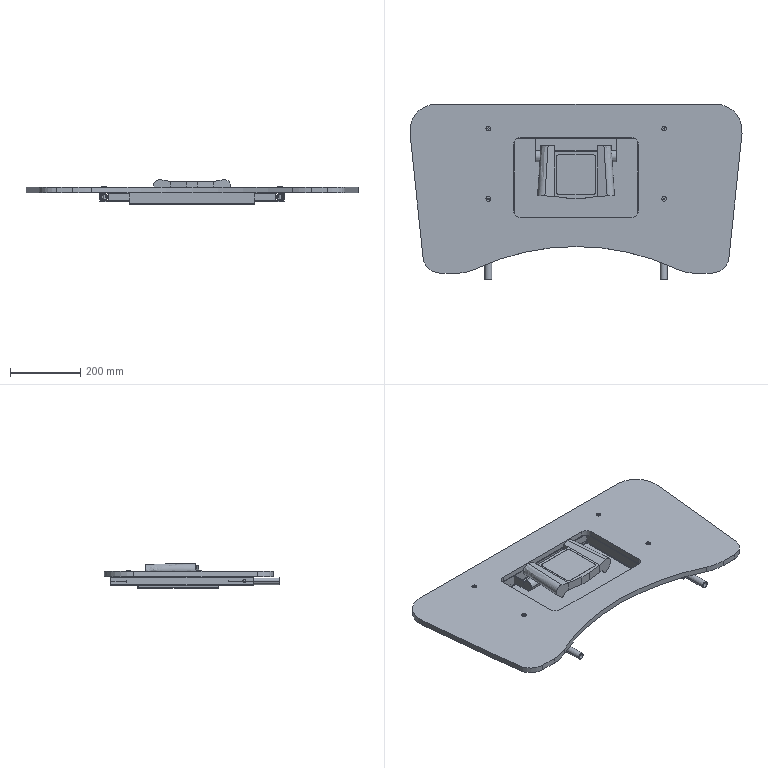Part | NX | features BREP 11 | 23 solids | 404 faces | box 948.321 x 501.65 x 70.752 mm | volume 6511824 mm3 | plane 199 | cylinder 127 | cone 52 | spline 14 | sphere 12 | commonest cylinder face diameters 4.826 x24 3.175 x18 9.525 x12 6.35 x8 6.604 x8 6.172 x6